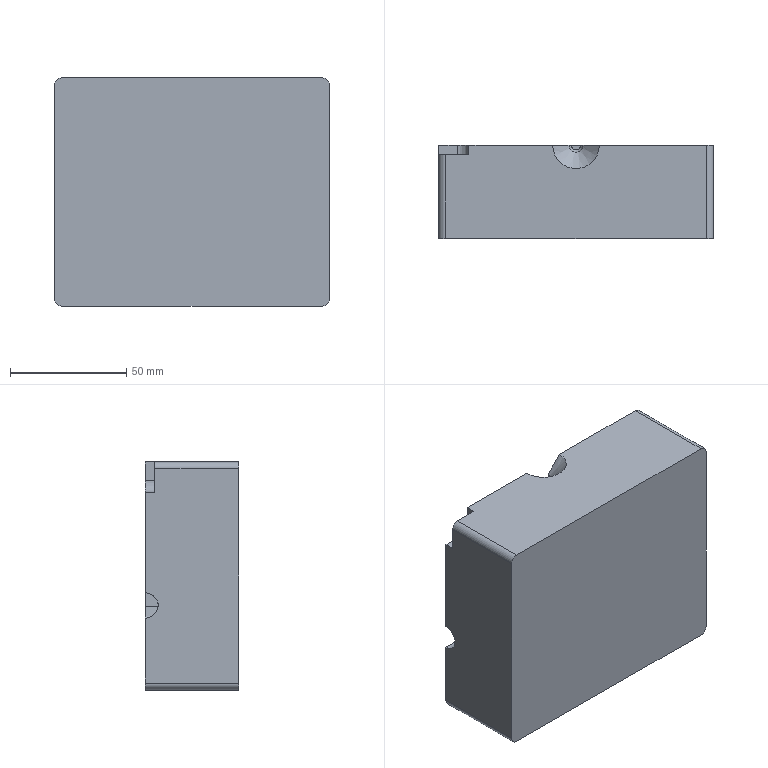Part | 1 solid | 92 faces | box 118 x 40 x 98 mm | volume 425542 mm3 | cylinder 35 | plane 32 | spline 12 | torus 11 | cone 1 | sphere 1 | commonest cylinder face diameters 6 x5 11.8 x4 2.472 x3 2.06 x2 3.09 x2 4.12 x2